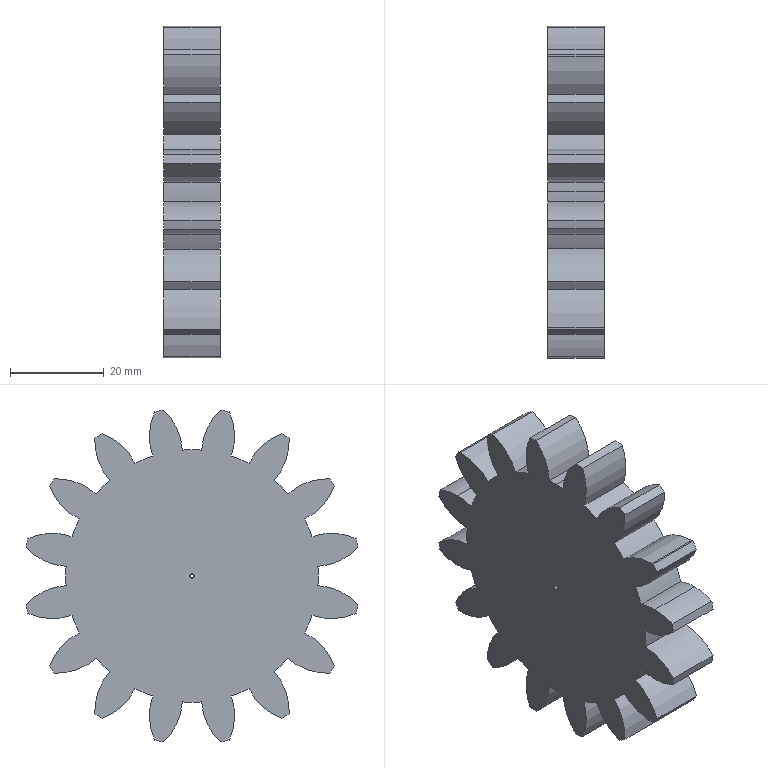Part | NX | 1 solid | 73 faces | box 12 x 70.969 x 70.969 mm | volume 36930 mm3 | cylinder 71 | plane 2 | commonest cylinder face diameters 25.6 x36 53.998 x17 72 x16 0.9 x2